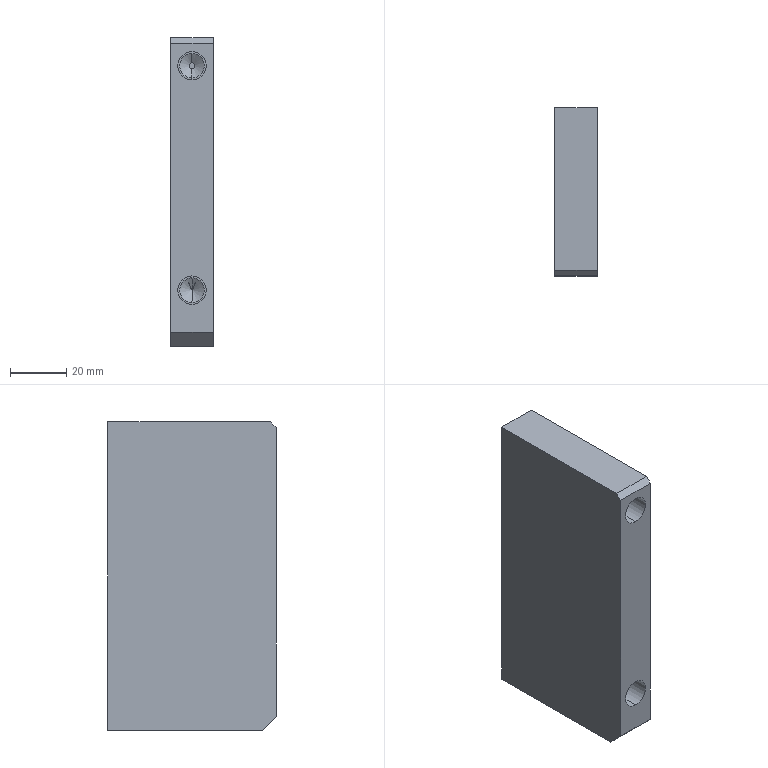Part | SolidWorks | features BaseBody 1 | 1 solid | 23 faces | box 15 x 60 x 110 mm | volume 93137 mm3 | plane 11 | cylinder 8 | cone 4 | commonest cylinder face diameters 8.8 x4 10.1 x4
STEP:
#1=CARTESIAN_POINT('',(-257.5,55.,208.171));
#2=VERTEX_POINT('',#1);
#3=CARTESIAN_POINT('',(-257.5,55.,198.071));
#4=VERTEX_POINT('',#3);
#5=CARTESIAN_POINT('',(-257.5,55.,203.121));
#6=DIRECTION('',(0.,-1.,0.));
#7=DIRECTION('',(0.,0.,-1.));
#8=AXIS2_PLACEMENT_3D('',#5,#6,#7);
#9=CIRCLE('',#8,5.05);
#10=EDGE_CURVE('',#2,#4,#9,.T.);
#11=ORIENTED_EDGE('',*,*,#10,.F.);
#12=CARTESIAN_POINT('',(-257.5,47.,208.171));
#13=VERTEX_POINT('',#12);
#14=CARTESIAN_POINT('',(-257.5,55.,208.171));
#15=DIRECTION('',(0.,-1.,0.));
#16=VECTOR('',#15,1000.);
#17=LINE('',#14,#16);
#18=EDGE_CURVE('',#2,#13,#17,.T.);
#19=ORIENTED_EDGE('',*,*,#18,.T.);
#20=CARTESIAN_POINT('',(-257.5,47.,198.071));
#21=VERTEX_POINT('',#20);
#22=CARTESIAN_POINT('',(-257.5,47.,203.121));
#23=DIRECTION('',(0.,-1.,0.));
#24=DIRECTION('',(0.,0.,-1.));
#25=AXIS2_PLACEMENT_3D('',#22,#23,#24);
#26=CIRCLE('',#25,5.05);
#27=EDGE_CURVE('',#13,#21,#26,.T.);
#28=ORIENTED_EDGE('',*,*,#27,.T.);
#29=CARTESIAN_POINT('',(-257.5,55.,198.071));
#30=DIRECTION('',(0.,-1.,0.));
#31=VECTOR('',#30,1000.);
#32=LINE('',#29,#31);
#33=EDGE_CURVE('',#4,#21,#32,.T.);
#34=ORIENTED_EDGE('',*,*,#33,.F.);
#35=EDGE_LOOP('',(#11,#19,#28,#34));
#36=FACE_OUTER_BOUND('',#35,.T.);
#37=CARTESIAN_POINT('',(-257.5,55.,203.121));
#38=DIRECTION('',(0.,-1.,0.));
#39=DIRECTION('',(0.,0.,-1.));
#40=AXIS2_PLACEMENT_3D('',#37,#38,#39);
#41=CYLINDRICAL_SURFACE('',#40,5.05);
#42=ADVANCED_FACE('',(#36),#41,.F.);
#43=CARTESIAN_POINT('',(-257.5,55.,128.171));
#44=VERTEX_POINT('',#43);
#45=CARTESIAN_POINT('',(-257.5,55.,118.071));
#46=VERTEX_POINT('',#45);
#47=CARTESIAN_POINT('',(-257.5,55.,123.121));
#48=DIRECTION('',(0.,-1.,0.));
#49=DIRECTION('',(0.,0.,-1.));
#50=AXIS2_PLACEMENT_3D('',#47,#48,#49);
#51=CIRCLE('',#50,5.05);
#52=EDGE_CURVE('',#44,#46,#51,.T.);
#53=ORIENTED_EDGE('',*,*,#52,.F.);
#54=CARTESIAN_POINT('',(-257.5,47.,128.171));
#55=VERTEX_POINT('',#54);
#56=CARTESIAN_POINT('',(-257.5,55.,128.171));
#57=DIRECTION('',(0.,-1.,0.));
#58=VECTOR('',#57,1000.);
#59=LINE('',#56,#58);
#60=EDGE_CURVE('',#44,#55,#59,.T.);
#61=ORIENTED_EDGE('',*,*,#60,.T.);
#62=CARTESIAN_POINT('',(-257.5,47.,118.071));
#63=VERTEX_POINT('',#62);
#64=CARTESIAN_POINT('',(-257.5,47.,123.121));
#65=DIRECTION('',(0.,-1.,0.));
#66=DIRECTION('',(0.,0.,-1.));
#67=AXIS2_PLACEMENT_3D('',#64,#65,#66);
#68=CIRCLE('',#67,5.05);
#69=EDGE_CURVE('',#55,#63,#68,.T.);
#70=ORIENTED_EDGE('',*,*,#69,.T.);
#71=CARTESIAN_POINT('',(-257.5,55.,118.071));
#72=DIRECTION('',(0.,-1.,0.));
#73=VECTOR('',#72,1000.);
#74=LINE('',#71,#73);
#75=EDGE_CURVE('',#46,#63,#74,.T.);
#76=ORIENTED_EDGE('',*,*,#75,.F.);
#77=EDGE_LOOP('',(#53,#61,#70,#76));
#78=FACE_OUTER_BOUND('',#77,.T.);
#79=CARTESIAN_POINT('',(-257.5,55.,123.121));
#80=DIRECTION('',(0.,-1.,0.));
#81=DIRECTION('',(0.,0.,-1.));
#82=AXIS2_PLACEMENT_3D('',#79,#80,#81);
#83=CYLINDRICAL_SURFACE('',#82,5.05);
#84=ADVANCED_FACE('',(#78),#83,.F.);
#85=CARTESIAN_POINT('',(-257.5,90.,207.521));
#86=VERTEX_POINT('',#85);
#87=CARTESIAN_POINT('',(-257.5,90.,198.721));
#88=VERTEX_POINT('',#87);
#89=CARTESIAN_POINT('',(-257.5,90.,203.121));
#90=DIRECTION('',(0.,-1.,0.));
#91=DIRECTION('',(0.,0.,-1.));
#92=AXIS2_PLACEMENT_3D('',#89,#90,#91);
#93=CIRCLE('',#92,4.4);
#94=EDGE_CURVE('',#86,#88,#93,.T.);
#95=ORIENTED_EDGE('',*,*,#94,.F.);
#96=CARTESIAN_POINT('',(-257.5,55.,207.521));
#97=VERTEX_POINT('',#96);
#98=CARTESIAN_POINT('',(-257.5,55.,207.521));
#99=DIRECTION('',(0.,-1.,0.));
#100=VECTOR('',#99,1000.);
#101=LINE('',#98,#100);
#102=EDGE_CURVE('',#86,#97,#101,.T.);
#103=ORIENTED_EDGE('',*,*,#102,.T.);
#104=CARTESIAN_POINT('',(-257.5,55.,198.721));
#105=VERTEX_POINT('',#104);
#106=CARTESIAN_POINT('',(-257.5,55.,203.121));
#107=DIRECTION('',(0.,1.,0.));
#108=DIRECTION('',(0.,0.,-1.));
#109=AXIS2_PLACEMENT_3D('',#106,#107,#108);
#110=CIRCLE('',#109,4.4);
#111=EDGE_CURVE('',#105,#97,#110,.T.);
#112=ORIENTED_EDGE('',*,*,#111,.F.);
#113=CARTESIAN_POINT('',(-257.5,55.,198.721));
#114=DIRECTION('',(0.,-1.,0.));
#115=VECTOR('',#114,1000.);
#116=LINE('',#113,#115);
#117=EDGE_CURVE('',#88,#105,#116,.T.);
#118=ORIENTED_EDGE('',*,*,#117,.F.);
#119=EDGE_LOOP('',(#95,#103,#112,#118));
#120=FACE_OUTER_BOUND('',#119,.T.);
#121=CARTESIAN_POINT('',(-257.5,55.,203.121));
#122=DIRECTION('',(0.,-1.,0.));
#123=DIRECTION('',(0.,0.,-1.));
#124=AXIS2_PLACEMENT_3D('',#121,#122,#123);
#125=CYLINDRICAL_SURFACE('',#124,4.4);
#126=ADVANCED_FACE('',(#120),#125,.F.);
#127=CARTESIAN_POINT('',(-257.5,90.,127.521));
#128=VERTEX_POINT('',#127);
#129=CARTESIAN_POINT('',(-257.5,90.,118.721));
#130=VERTEX_POINT('',#129);
#131=CARTESIAN_POINT('',(-257.5,90.,123.121));
#132=DIRECTION('',(0.,-1.,0.));
#133=DIRECTION('',(0.,0.,-1.));
#134=AXIS2_PLACEMENT_3D('',#131,#132,#133);
#135=CIRCLE('',#134,4.4);
#136=EDGE_CURVE('',#128,#130,#135,.T.);
#137=ORIENTED_EDGE('',*,*,#136,.F.);
#138=CARTESIAN_POINT('',(-257.5,55.,127.521));
#139=VERTEX_POINT('',#138);
#140=CARTESIAN_POINT('',(-257.5,55.,127.521));
#141=DIRECTION('',(0.,-1.,0.));
#142=VECTOR('',#141,1000.);
#143=LINE('',#140,#142);
#144=EDGE_CURVE('',#128,#139,#143,.T.);
#145=ORIENTED_EDGE('',*,*,#144,.T.);
#146=CARTESIAN_POINT('',(-257.5,55.,118.721));
#147=VERTEX_POINT('',#146);
#148=CARTESIAN_POINT('',(-257.5,55.,123.121));
#149=DIRECTION('',(0.,1.,0.));
#150=DIRECTION('',(0.,0.,-1.));
#151=AXIS2_PLACEMENT_3D('',#148,#149,#150);
#152=CIRCLE('',#151,4.4);
#153=EDGE_CURVE('',#147,#139,#152,.T.);
#154=ORIENTED_EDGE('',*,*,#153,.F.);
#155=CARTESIAN_POINT('',(-257.5,55.,118.721));
#156=DIRECTION('',(0.,-1.,0.));
#157=VECTOR('',#156,1000.);
#158=LINE('',#155,#157);
#159=EDGE_CURVE('',#130,#147,#158,.T.);
#160=ORIENTED_EDGE('',*,*,#159,.F.);
#161=EDGE_LOOP('',(#137,#145,#154,#160));
#162=FACE_OUTER_BOUND('',#161,.T.);
#163=CARTESIAN_POINT('',(-257.5,55.,123.121));
#164=DIRECTION('',(0.,-1.,0.));
#165=DIRECTION('',(0.,0.,-1.));
#166=AXIS2_PLACEMENT_3D('',#163,#164,#165);
#167=CYLINDRICAL_SURFACE('',#166,4.4);
#168=ADVANCED_FACE('',(#162),#167,.F.);
#169=CARTESIAN_POINT('',(-257.5,92.,204.193));
#170=VERTEX_POINT('',#169);
#171=CARTESIAN_POINT('',(-257.5,92.,202.05));
#172=VERTEX_POINT('',#171);
#173=CARTESIAN_POINT('',(-257.5,92.,203.121));
#174=DIRECTION('',(0.,-1.,0.));
#175=DIRECTION('',(0.,0.,-1.));
#176=AXIS2_PLACEMENT_3D('',#173,#174,#175);
#177=CIRCLE('',#176,1.071);
#178=EDGE_CURVE('',#170,#172,#177,.T.);
#179=ORIENTED_EDGE('',*,*,#178,.F.);
#180=CARTESIAN_POINT('',(-257.5,90.,207.521));
#181=DIRECTION('',(0.,-0.515,0.8572));
#182=VECTOR('',#181,1000.);
#183=LINE('',#180,#182);
#184=EDGE_CURVE('',#170,#86,#183,.T.);
#185=ORIENTED_EDGE('',*,*,#184,.T.);
#186=ORIENTED_EDGE('',*,*,#94,.T.);
#187=CARTESIAN_POINT('',(-257.5,90.,198.721));
#188=DIRECTION('',(0.,-0.515,-0.8572));
#189=VECTOR('',#188,1000.);
#190=LINE('',#187,#189);
#191=EDGE_CURVE('',#172,#88,#190,.T.);
#192=ORIENTED_EDGE('',*,*,#191,.F.);
#193=EDGE_LOOP('',(#179,#185,#186,#192));
#194=FACE_OUTER_BOUND('',#193,.T.);
#195=CARTESIAN_POINT('',(-257.5,90.,203.121));
#196=DIRECTION('',(0.,-1.,0.));
#197=DIRECTION('',(0.,0.,-1.));
#198=AXIS2_PLACEMENT_3D('',#195,#196,#197);
#199=CONICAL_SURFACE('',#198,4.4,1.03);
#200=ADVANCED_FACE('',(#194),#199,.F.);
#201=CARTESIAN_POINT('',(-257.5,92.644,123.121));
#202=VERTEX_POINT('',#201);
#203=CARTESIAN_POINT('',(-257.5,90.,118.721));
#204=DIRECTION('',(0.,-0.515,-0.8572));
#205=VECTOR('',#204,1000.);
#206=LINE('',#203,#205);
#207=EDGE_CURVE('',#202,#130,#206,.T.);
#208=ORIENTED_EDGE('',*,*,#207,.F.);
#209=CARTESIAN_POINT('',(-257.5,90.,127.521));
#210=DIRECTION('',(0.,-0.515,0.8572));
#211=VECTOR('',#210,1000.);
#212=LINE('',#209,#211);
#213=EDGE_CURVE('',#202,#128,#212,.T.);
#214=ORIENTED_EDGE('',*,*,#213,.T.);
#215=ORIENTED_EDGE('',*,*,#136,.T.);
#216=EDGE_LOOP('',(#208,#214,#215));
#217=FACE_OUTER_BOUND('',#216,.T.);
#218=CARTESIAN_POINT('',(-257.5,90.,123.121));
#219=DIRECTION('',(0.,-1.,0.));
#220=DIRECTION('',(0.,0.,-1.));
#221=AXIS2_PLACEMENT_3D('',#218,#219,#220);
#222=CONICAL_SURFACE('',#221,4.4,1.03);
#223=ADVANCED_FACE('',(#217),#222,.F.);
#224=CARTESIAN_POINT('',(-265.,52.,103.121));
#225=VERTEX_POINT('',#224);
#226=CARTESIAN_POINT('',(-265.,107.,103.121));
#227=VERTEX_POINT('',#226);
#228=CARTESIAN_POINT('',(-265.,47.,103.121));
#229=DIRECTION('',(0.,1.,0.));
#230=VECTOR('',#229,1000.);
#231=LINE('',#228,#230);
#232=EDGE_CURVE('',#225,#227,#231,.T.);
#233=ORIENTED_EDGE('',*,*,#232,.F.);
#234=CARTESIAN_POINT('',(-265.,47.,108.121));
#235=VERTEX_POINT('',#234);
#236=CARTESIAN_POINT('',(-265.,47.,108.121));
#237=DIRECTION('',(0.,0.7071,-0.7071));
#238=VECTOR('',#237,1000.);
#239=LINE('',#236,#238);
#240=EDGE_CURVE('',#235,#225,#239,.T.);
#241=ORIENTED_EDGE('',*,*,#240,.F.);
#242=CARTESIAN_POINT('',(-265.,47.,211.121));
#243=VERTEX_POINT('',#242);
#244=CARTESIAN_POINT('',(-265.,47.,103.121));
#245=DIRECTION('',(0.,0.,-1.));
#246=VECTOR('',#245,1000.);
#247=LINE('',#244,#246);
#248=EDGE_CURVE('',#243,#235,#247,.T.);
#249=ORIENTED_EDGE('',*,*,#248,.F.);
#250=CARTESIAN_POINT('',(-265.,49.,213.121));
#251=VERTEX_POINT('',#250);
#252=CARTESIAN_POINT('',(-265.,49.,213.121));
#253=DIRECTION('',(0.,-0.7071,-0.7071));
#254=VECTOR('',#253,1000.);
#255=LINE('',#252,#254);
#256=EDGE_CURVE('',#251,#243,#255,.T.);
#257=ORIENTED_EDGE('',*,*,#256,.F.);
#258=CARTESIAN_POINT('',(-265.,107.,213.121));
#259=VERTEX_POINT('',#258);
#260=CARTESIAN_POINT('',(-265.,47.,213.121));
#261=DIRECTION('',(0.,-1.,0.));
#262=VECTOR('',#261,1000.);
#263=LINE('',#260,#262);
#264=EDGE_CURVE('',#259,#251,#263,.T.);
#265=ORIENTED_EDGE('',*,*,#264,.F.);
#266=CARTESIAN_POINT('',(-265.,107.,103.121));
#267=DIRECTION('',(0.,0.,1.));
#268=VECTOR('',#267,1000.);
#269=LINE('',#266,#268);
#270=EDGE_CURVE('',#227,#259,#269,.T.);
#271=ORIENTED_EDGE('',*,*,#270,.F.);
#272=EDGE_LOOP('',(#233,#241,#249,#257,#265,#271));
#273=FACE_OUTER_BOUND('',#272,.T.);
#274=CARTESIAN_POINT('',(-265.,47.,103.121));
#275=DIRECTION('',(1.,0.,0.));
#276=DIRECTION('',(0.,0.,-1.));
#277=AXIS2_PLACEMENT_3D('',#274,#275,#276);
#278=PLANE('',#277);
#279=ADVANCED_FACE('',(#273),#278,.F.);
#280=CARTESIAN_POINT('',(-250.,107.,103.121));
#281=VERTEX_POINT('',#280);
#282=CARTESIAN_POINT('',(-337.5,107.,103.121));
#283=DIRECTION('',(1.,0.,0.));
#284=VECTOR('',#283,1000.);
#285=LINE('',#282,#284);
#286=EDGE_CURVE('',#227,#281,#285,.T.);
#287=ORIENTED_EDGE('',*,*,#286,.F.);
#288=ORIENTED_EDGE('',*,*,#270,.T.);
#289=CARTESIAN_POINT('',(-250.,107.,213.121));
#290=VERTEX_POINT('',#289);
#291=CARTESIAN_POINT('',(-337.5,107.,213.121));
#292=DIRECTION('',(-1.,0.,0.));
#293=VECTOR('',#292,1000.);
#294=LINE('',#291,#293);
#295=EDGE_CURVE('',#290,#259,#294,.T.);
#296=ORIENTED_EDGE('',*,*,#295,.F.);
#297=CARTESIAN_POINT('',(-250.,107.,153.121));
#298=DIRECTION('',(0.,0.,1.));
#299=VECTOR('',#298,1000.);
#300=LINE('',#297,#299);
#301=EDGE_CURVE('',#281,#290,#300,.T.);
#302=ORIENTED_EDGE('',*,*,#301,.F.);
#303=EDGE_LOOP('',(#287,#288,#296,#302));
#304=FACE_OUTER_BOUND('',#303,.T.);
#305=CARTESIAN_POINT('',(-337.5,107.,153.121));
#306=DIRECTION('',(0.,-1.,0.));
#307=DIRECTION('',(0.,0.,-1.));
#308=AXIS2_PLACEMENT_3D('',#305,#306,#307);
#309=PLANE('',#308);
#310=ADVANCED_FACE('',(#304),#309,.F.);
#311=ORIENTED_EDGE('',*,*,#286,.T.);
#312=CARTESIAN_POINT('',(-250.,52.,103.121));
#313=VERTEX_POINT('',#312);
#314=CARTESIAN_POINT('',(-250.,92.,103.121));
#315=DIRECTION('',(0.,1.,0.));
#316=VECTOR('',#315,1000.);
#317=LINE('',#314,#316);
#318=EDGE_CURVE('',#313,#281,#317,.T.);
#319=ORIENTED_EDGE('',*,*,#318,.F.);
#320=CARTESIAN_POINT('',(-425.,52.,103.121));
#321=DIRECTION('',(1.,0.,0.));
#322=VECTOR('',#321,1000.);
#323=LINE('',#320,#322);
#324=EDGE_CURVE('',#225,#313,#323,.T.);
#325=ORIENTED_EDGE('',*,*,#324,.F.);
#326=ORIENTED_EDGE('',*,*,#232,.T.);
#327=EDGE_LOOP('',(#311,#319,#325,#326));
#328=FACE_OUTER_BOUND('',#327,.T.);
#329=CARTESIAN_POINT('',(-425.,92.,103.121));
#330=DIRECTION('',(0.,0.,1.));
#331=DIRECTION('',(1.,0.,0.));
#332=AXIS2_PLACEMENT_3D('',#329,#330,#331);
#333=PLANE('',#332);
#334=ADVANCED_FACE('',(#328),#333,.F.);
#335=ORIENTED_EDGE('',*,*,#324,.T.);
#336=CARTESIAN_POINT('',(-250.,47.,108.121));
#337=VERTEX_POINT('',#336);
#338=CARTESIAN_POINT('',(-250.,47.,108.121));
#339=DIRECTION('',(0.,0.7071,-0.7071));
#340=VECTOR('',#339,1000.);
#341=LINE('',#338,#340);
#342=EDGE_CURVE('',#337,#313,#341,.T.);
#343=ORIENTED_EDGE('',*,*,#342,.F.);
#344=CARTESIAN_POINT('',(-337.5,47.,108.121));
#345=DIRECTION('',(1.,0.,0.));
#346=VECTOR('',#345,1000.);
#347=LINE('',#344,#346);
#348=EDGE_CURVE('',#235,#337,#347,.T.);
#349=ORIENTED_EDGE('',*,*,#348,.F.);
#350=ORIENTED_EDGE('',*,*,#240,.T.);
#351=EDGE_LOOP('',(#335,#343,#349,#350));
#352=FACE_OUTER_BOUND('',#351,.T.);
#353=CARTESIAN_POINT('',(-337.5,47.,108.121));
#354=DIRECTION('',(0.,0.7071,0.7071));
#355=DIRECTION('',(0.,-0.7071,0.7071));
#356=AXIS2_PLACEMENT_3D('',#353,#354,#355);
#357=PLANE('',#356);
#358=ADVANCED_FACE('',(#352),#357,.F.);
#359=CARTESIAN_POINT('',(-250.,47.,211.121));
#360=VERTEX_POINT('',#359);
#361=CARTESIAN_POINT('',(-337.5,47.,211.121));
#362=DIRECTION('',(1.,0.,0.));
#363=VECTOR('',#362,1000.);
#364=LINE('',#361,#363);
#365=EDGE_CURVE('',#243,#360,#364,.T.);
#366=ORIENTED_EDGE('',*,*,#365,.F.);
#367=ORIENTED_EDGE('',*,*,#248,.T.);
#368=ORIENTED_EDGE('',*,*,#348,.T.);
#369=CARTESIAN_POINT('',(-250.,47.,153.121));
#370=DIRECTION('',(0.,0.,-1.));
#371=VECTOR('',#370,1000.);
#372=LINE('',#369,#371);
#373=EDGE_CURVE('',#360,#337,#372,.T.);
#374=ORIENTED_EDGE('',*,*,#373,.F.);
#375=EDGE_LOOP('',(#366,#367,#368,#374));
#376=FACE_OUTER_BOUND('',#375,.T.);
#377=CARTESIAN_POINT('',(-257.5,47.,203.121));
#378=DIRECTION('',(0.,-1.,0.));
#379=DIRECTION('',(0.,0.,-1.));
#380=AXIS2_PLACEMENT_3D('',#377,#378,#379);
#381=CIRCLE('',#380,5.05);
#382=EDGE_CURVE('',#21,#13,#381,.T.);
#383=ORIENTED_EDGE('',*,*,#382,.F.);
#384=ORIENTED_EDGE('',*,*,#27,.F.);
#385=EDGE_LOOP('',(#383,#384));
#386=FACE_BOUND('',#385,.T.);
#387=CARTESIAN_POINT('',(-257.5,47.,123.121));
#388=DIRECTION('',(0.,-1.,0.));
#389=DIRECTION('',(0.,0.,-1.));
#390=AXIS2_PLACEMENT_3D('',#387,#388,#389);
#391=CIRCLE('',#390,5.05);
#392=EDGE_CURVE('',#63,#55,#391,.T.);
#393=ORIENTED_EDGE('',*,*,#392,.F.);
#394=ORIENTED_EDGE('',*,*,#69,.F.);
#395=EDGE_LOOP('',(#393,#394));
#396=FACE_BOUND('',#395,.T.);
#397=CARTESIAN_POINT('',(-337.5,47.,153.121));
#398=DIRECTION('',(0.,1.,0.));
#399=DIRECTION('',(0.,0.,1.));
#400=AXIS2_PLACEMENT_3D('',#397,#398,#399);
#401=PLANE('',#400);
#402=ADVANCED_FACE('',(#376,#386,#396),#401,.F.);
#403=CARTESIAN_POINT('',(-250.,49.,213.121));
#404=VERTEX_POINT('',#403);
#405=CARTESIAN_POINT('',(-250.,49.,213.121));
#406=DIRECTION('',(0.,0.7071,0.7071));
#407=VECTOR('',#406,1000.);
#408=LINE('',#405,#407);
#409=EDGE_CURVE('',#360,#404,#408,.T.);
#410=ORIENTED_EDGE('',*,*,#409,.T.);
#411=CARTESIAN_POINT('',(-337.5,49.,213.121));
#412=DIRECTION('',(-1.,0.,0.));
#413=VECTOR('',#412,1000.);
#414=LINE('',#411,#413);
#415=EDGE_CURVE('',#404,#251,#414,.T.);
#416=ORIENTED_EDGE('',*,*,#415,.T.);
#417=ORIENTED_EDGE('',*,*,#256,.T.);
#418=ORIENTED_EDGE('',*,*,#365,.T.);
#419=EDGE_LOOP('',(#410,#416,#417,#418));
#420=FACE_OUTER_BOUND('',#419,.T.);
#421=CARTESIAN_POINT('',(-337.5,49.,213.121));
#422=DIRECTION('',(0.,-0.7071,0.7071));
#423=DIRECTION('',(0.,-0.7071,-0.7071));
#424=AXIS2_PLACEMENT_3D('',#421,#422,#423);
#425=PLANE('',#424);
#426=ADVANCED_FACE('',(#420),#425,.T.);
#427=ORIENTED_EDGE('',*,*,#264,.T.);
#428=ORIENTED_EDGE('',*,*,#415,.F.);
#429=CARTESIAN_POINT('',(-250.,107.,213.121));
#430=DIRECTION('',(0.,1.,0.));
#431=VECTOR('',#430,1000.);
#432=LINE('',#429,#431);
#433=EDGE_CURVE('',#404,#290,#432,.T.);
#434=ORIENTED_EDGE('',*,*,#433,.T.);
#435=ORIENTED_EDGE('',*,*,#295,.T.);
#436=EDGE_LOOP('',(#427,#428,#434,#435));
#437=FACE_OUTER_BOUND('',#436,.T.);
#438=CARTESIAN_POINT('',(-337.5,107.,213.121));
#439=DIRECTION('',(0.,0.,1.));
#440=DIRECTION('',(1.,0.,0.));
#441=AXIS2_PLACEMENT_3D('',#438,#439,#440);
#442=PLANE('',#441);
#443=ADVANCED_FACE('',(#437),#442,.T.);
#444=ORIENTED_EDGE('',*,*,#301,.T.);
#445=ORIENTED_EDGE('',*,*,#433,.F.);
#446=ORIENTED_EDGE('',*,*,#409,.F.);
#447=ORIENTED_EDGE('',*,*,#373,.T.);
#448=ORIENTED_EDGE('',*,*,#342,.T.);
#449=ORIENTED_EDGE('',*,*,#318,.T.);
#450=EDGE_LOOP('',(#444,#445,#446,#447,#448,#449));
#451=FACE_OUTER_BOUND('',#450,.T.);
#452=CARTESIAN_POINT('',(-250.,92.,103.121));
#453=DIRECTION('',(-1.,0.,0.));
#454=DIRECTION('',(0.,0.,1.));
#455=AXIS2_PLACEMENT_3D('',#452,#453,#454);
#456=PLANE('',#455);
#457=ADVANCED_FACE('',(#451),#456,.F.);
#458=ORIENTED_EDGE('',*,*,#18,.F.);
#459=CARTESIAN_POINT('',(-257.5,55.,203.121));
#460=DIRECTION('',(0.,-1.,0.));
#461=DIRECTION('',(0.,0.,-1.));
#462=AXIS2_PLACEMENT_3D('',#459,#460,#461);
#463=CIRCLE('',#462,5.05);
#464=EDGE_CURVE('',#4,#2,#463,.T.);
#465=ORIENTED_EDGE('',*,*,#464,.F.);
#466=ORIENTED_EDGE('',*,*,#33,.T.);
#467=ORIENTED_EDGE('',*,*,#382,.T.);
#468=EDGE_LOOP('',(#458,#465,#466,#467));
#469=FACE_OUTER_BOUND('',#468,.T.);
#470=CARTESIAN_POINT('',(-257.5,55.,203.121));
#471=DIRECTION('',(0.,-1.,0.));
#472=DIRECTION('',(0.,0.,-1.));
#473=AXIS2_PLACEMENT_3D('',#470,#471,#472);
#474=CYLINDRICAL_SURFACE('',#473,5.05);
#475=ADVANCED_FACE('',(#469),#474,.F.);
#476=ORIENTED_EDGE('',*,*,#60,.F.);
#477=CARTESIAN_POINT('',(-257.5,55.,123.121));
#478=DIRECTION('',(0.,-1.,0.));
#479=DIRECTION('',(0.,0.,-1.));
#480=AXIS2_PLACEMENT_3D('',#477,#478,#479);
#481=CIRCLE('',#480,5.05);
#482=EDGE_CURVE('',#46,#44,#481,.T.);
#483=ORIENTED_EDGE('',*,*,#482,.F.);
#484=ORIENTED_EDGE('',*,*,#75,.T.);
#485=ORIENTED_EDGE('',*,*,#392,.T.);
#486=EDGE_LOOP('',(#476,#483,#484,#485));
#487=FACE_OUTER_BOUND('',#486,.T.);
#488=CARTESIAN_POINT('',(-257.5,55.,123.121));
#489=DIRECTION('',(0.,-1.,0.));
#490=DIRECTION('',(0.,0.,-1.));
#491=AXIS2_PLACEMENT_3D('',#488,#489,#490);
#492=CYLINDRICAL_SURFACE('',#491,5.05);
#493=ADVANCED_FACE('',(#487),#492,.F.);
#494=ORIENTED_EDGE('',*,*,#464,.T.);
#495=ORIENTED_EDGE('',*,*,#10,.T.);
#496=EDGE_LOOP('',(#494,#495));
#497=FACE_OUTER_BOUND('',#496,.T.);
#498=ORIENTED_EDGE('',*,*,#111,.T.);
#499=CARTESIAN_POINT('',(-257.5,55.,203.121));
#500=DIRECTION('',(0.,1.,0.));
#501=DIRECTION('',(0.,0.,-1.));
#502=AXIS2_PLACEMENT_3D('',#499,#500,#501);
#503=CIRCLE('',#502,4.4);
#504=EDGE_CURVE('',#97,#105,#503,.T.);
#505=ORIENTED_EDGE('',*,*,#504,.T.);
#506=EDGE_LOOP('',(#498,#505));
#507=FACE_BOUND('',#506,.T.);
#508=CARTESIAN_POINT('',(-257.5,55.,203.121));
#509=DIRECTION('',(0.,-1.,0.));
#510=DIRECTION('',(0.,0.,-1.));
#511=AXIS2_PLACEMENT_3D('',#508,#509,#510);
#512=PLANE('',#511);
#513=ADVANCED_FACE('',(#497,#507),#512,.T.);
#514=ORIENTED_EDGE('',*,*,#482,.T.);
#515=ORIENTED_EDGE('',*,*,#52,.T.);
#516=EDGE_LOOP('',(#514,#515));
#517=FACE_OUTER_BOUND('',#516,.T.);
#518=ORIENTED_EDGE('',*,*,#153,.T.);
#519=CARTESIAN_POINT('',(-257.5,55.,123.121));
#520=DIRECTION('',(0.,1.,0.));
#521=DIRECTION('',(0.,0.,-1.));
#522=AXIS2_PLACEMENT_3D('',#519,#520,#521);
#523=CIRCLE('',#522,4.4);
#524=EDGE_CURVE('',#139,#147,#523,.T.);
#525=ORIENTED_EDGE('',*,*,#524,.T.);
#526=EDGE_LOOP('',(#518,#525));
#527=FACE_BOUND('',#526,.T.);
#528=CARTESIAN_POINT('',(-257.5,55.,123.121));
#529=DIRECTION('',(0.,-1.,0.));
#530=DIRECTION('',(0.,0.,-1.));
#531=AXIS2_PLACEMENT_3D('',#528,#529,#530);
#532=PLANE('',#531);
#533=ADVANCED_FACE('',(#517,#527),#532,.T.);
#534=ORIENTED_EDGE('',*,*,#102,.F.);
#535=CARTESIAN_POINT('',(-257.5,90.,203.121));
#536=DIRECTION('',(0.,-1.,0.));
#537=DIRECTION('',(0.,0.,-1.));
#538=AXIS2_PLACEMENT_3D('',#535,#536,#537);
#539=CIRCLE('',#538,4.4);
#540=EDGE_CURVE('',#88,#86,#539,.T.);
#541=ORIENTED_EDGE('',*,*,#540,.F.);
#542=ORIENTED_EDGE('',*,*,#117,.T.);
#543=ORIENTED_EDGE('',*,*,#504,.F.);
#544=EDGE_LOOP('',(#534,#541,#542,#543));
#545=FACE_OUTER_BOUND('',#544,.T.);
#546=CARTESIAN_POINT('',(-257.5,55.,203.121));
#547=DIRECTION('',(0.,-1.,0.));
#548=DIRECTION('',(0.,0.,-1.));
#549=AXIS2_PLACEMENT_3D('',#546,#547,#548);
#550=CYLINDRICAL_SURFACE('',#549,4.4);
#551=ADVANCED_FACE('',(#545),#550,.F.);
#552=ORIENTED_EDGE('',*,*,#144,.F.);
#553=CARTESIAN_POINT('',(-257.5,90.,123.121));
#554=DIRECTION('',(0.,-1.,0.));
#555=DIRECTION('',(0.,0.,-1.));
#556=AXIS2_PLACEMENT_3D('',#553,#554,#555);
#557=CIRCLE('',#556,4.4);
#558=EDGE_CURVE('',#130,#128,#557,.T.);
#559=ORIENTED_EDGE('',*,*,#558,.F.);
#560=ORIENTED_EDGE('',*,*,#159,.T.);
#561=ORIENTED_EDGE('',*,*,#524,.F.);
#562=EDGE_LOOP('',(#552,#559,#560,#561));
#563=FACE_OUTER_BOUND('',#562,.T.);
#564=CARTESIAN_POINT('',(-257.5,55.,123.121));
#565=DIRECTION('',(0.,-1.,0.));
#566=DIRECTION('',(0.,0.,-1.));
#567=AXIS2_PLACEMENT_3D('',#564,#565,#566);
#568=CYLINDRICAL_SURFACE('',#567,4.4);
#569=ADVANCED_FACE('',(#563),#568,.F.);
#570=ORIENTED_EDGE('',*,*,#184,.F.);
#571=CARTESIAN_POINT('',(-257.5,92.,203.121));
#572=DIRECTION('',(0.,-1.,0.));
#573=DIRECTION('',(0.,0.,-1.));
#574=AXIS2_PLACEMENT_3D('',#571,#572,#573);
#575=CIRCLE('',#574,1.071);
#576=EDGE_CURVE('',#172,#170,#575,.T.);
#577=ORIENTED_EDGE('',*,*,#576,.F.);
#578=ORIENTED_EDGE('',*,*,#191,.T.);
#579=ORIENTED_EDGE('',*,*,#540,.T.);
#580=EDGE_LOOP('',(#570,#577,#578,#579));
#581=FACE_OUTER_BOUND('',#580,.T.);
#582=CARTESIAN_POINT('',(-257.5,90.,203.121));
#583=DIRECTION('',(0.,-1.,0.));
#584=DIRECTION('',(0.,0.,-1.));
#585=AXIS2_PLACEMENT_3D('',#582,#583,#584);
#586=CONICAL_SURFACE('',#585,4.4,1.03);
#587=ADVANCED_FACE('',(#581),#586,.F.);
#588=ORIENTED_EDGE('',*,*,#213,.F.);
#589=ORIENTED_EDGE('',*,*,#207,.T.);
#590=ORIENTED_EDGE('',*,*,#558,.T.);
#591=EDGE_LOOP('',(#588,#589,#590));
#592=FACE_OUTER_BOUND('',#591,.T.);
#593=CARTESIAN_POINT('',(-257.5,90.,123.121));
#594=DIRECTION('',(0.,-1.,0.));
#595=DIRECTION('',(0.,0.,-1.));
#596=AXIS2_PLACEMENT_3D('',#593,#594,#595);
#597=CONICAL_SURFACE('',#596,4.4,1.03);
#598=ADVANCED_FACE('',(#592),#597,.F.);
#599=ORIENTED_EDGE('',*,*,#576,.T.);
#600=ORIENTED_EDGE('',*,*,#178,.T.);
#601=EDGE_LOOP('',(#599,#600));
#602=FACE_OUTER_BOUND('',#601,.T.);
#603=CARTESIAN_POINT('',(-395.863,92.,153.121));
#604=DIRECTION('',(0.,-1.,0.));
#605=DIRECTION('',(0.,0.,-1.));
#606=AXIS2_PLACEMENT_3D('',#603,#604,#605);
#607=PLANE('',#606);
#608=ADVANCED_FACE('',(#602),#607,.T.);
#609=CLOSED_SHELL('',(#42,#84,#126,#168,#200,#223,#279,#310,#334,#358,#402,#426,#443,#457,#475,#493,#513,#533,#551,#569,#587,#598,#608));
#610=MANIFOLD_SOLID_BREP('',#609);
#611=CARTESIAN_POINT('',(0.,0.,0.));
#612=DIRECTION('',(0.,0.,1.));
#613=DIRECTION('',(1.,0.,0.));
#614=AXIS2_PLACEMENT_3D('',#611,#612,#613);
#615=(LENGTH_UNIT()NAMED_UNIT(*)SI_UNIT(.MILLI.,.METRE.));
#616=UNCERTAINTY_MEASURE_WITH_UNIT(LENGTH_MEASURE(0.00001),#615,'','');
#617=(NAMED_UNIT(*)PLANE_ANGLE_UNIT()SI_UNIT($,.RADIAN.));
#618=(NAMED_UNIT(*)SI_UNIT($,.STERADIAN.)SOLID_ANGLE_UNIT());
#619=(GEOMETRIC_REPRESENTATION_CONTEXT(3)GLOBAL_UNCERTAINTY_ASSIGNED_CONTEXT((#616))GLOBAL_UNIT_ASSIGNED_CONTEXT((#615,#617,#618))REPRESENTATION_CONTEXT('',''));
#620=ADVANCED_BREP_SHAPE_REPRESENTATION('',(#610,#614),#619);